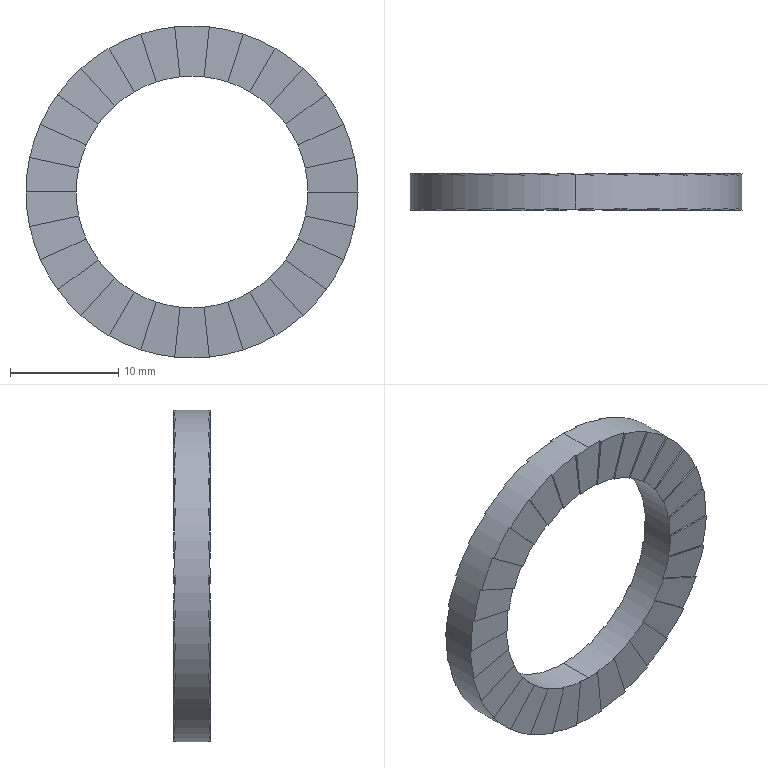Part | SolidWorks | features ICE 3, CirPattern 1, Extrusion 1, MirrorSolid 1 | 1 solid | 124 faces | box 30.7 x 3.4 x 30.7 mm | volume 1238 mm3 | plane 120 | cylinder 4 | commonest cylinder face diameters 21.4 x2 30.7 x2